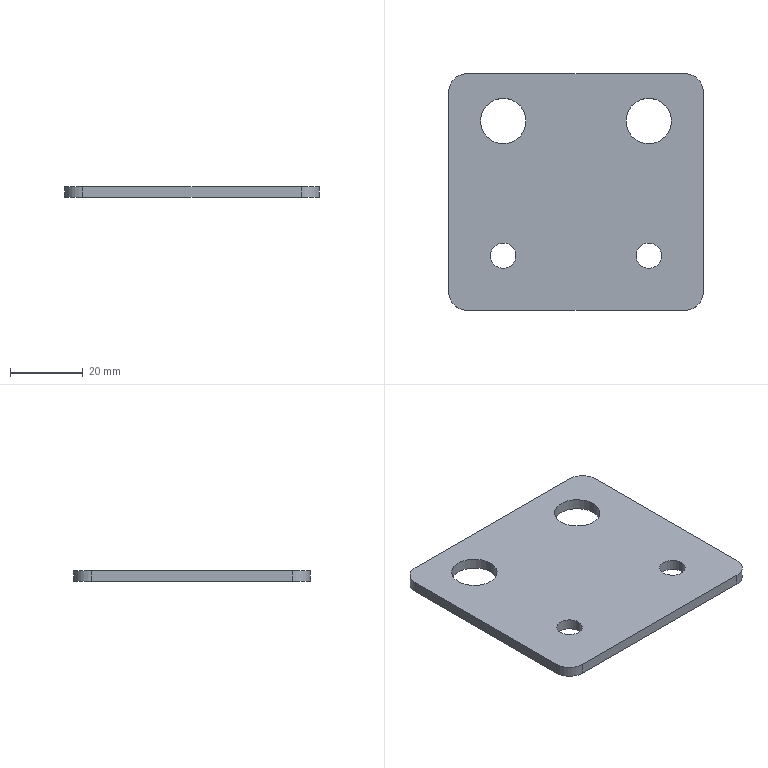Part | STEP file | Sensor mounting plate | 1 solid | 18 faces | box 70 x 65 x 3 mm | volume 12618 mm3 | cylinder 12 | plane 6 | commonest cylinder face diameters 7 x4 10 x4 12.5 x4
STEP:
#1=CARTESIAN_POINT('',(0.,0.,0.));
#2=DIRECTION('',(0.,0.,1.));
#3=DIRECTION('',(1.,0.,0.));
#4=AXIS2_PLACEMENT_3D('',#1,#2,#3);
#5=CARTESIAN_POINT('',(-16.5,-17.5,0.));
#6=VERTEX_POINT('',#5);
#7=CARTESIAN_POINT('',(-16.5,-17.5,3.));
#8=VERTEX_POINT('',#7);
#9=CARTESIAN_POINT('',(-16.5,-17.5,3.));
#10=DIRECTION('',(0.,0.,1.));
#11=VECTOR('',#10,1.);
#12=LINE('',#9,#11);
#13=CARTESIAN_POINT('',(-20.,-17.5,3.));
#14=DIRECTION('',(0.,0.,1.));
#15=DIRECTION('',(1.,0.,0.));
#16=AXIS2_PLACEMENT_3D('',#13,#14,#15);
#17=CYLINDRICAL_SURFACE('',#16,3.5);
#18=CARTESIAN_POINT('',(6.283,0.));
#19=DIRECTION('',(0.,1.));
#20=VECTOR('',#19,1.);
#21=LINE('',#18,#20);
#22=(GEOMETRIC_REPRESENTATION_CONTEXT(2)PARAMETRIC_REPRESENTATION_CONTEXT()REPRESENTATION_CONTEXT('',''));
#23=DEFINITIONAL_REPRESENTATION('',(#21),#22);
#24=PCURVE('',#17,#23);
#25=CARTESIAN_POINT('',(-20.,-17.5,3.));
#26=DIRECTION('',(0.,0.,1.));
#27=DIRECTION('',(1.,0.,0.));
#28=AXIS2_PLACEMENT_3D('',#25,#26,#27);
#29=CYLINDRICAL_SURFACE('',#28,3.5);
#30=CARTESIAN_POINT('',(0.,0.));
#31=DIRECTION('',(0.,1.));
#32=VECTOR('',#31,1.);
#33=LINE('',#30,#32);
#34=(GEOMETRIC_REPRESENTATION_CONTEXT(2)PARAMETRIC_REPRESENTATION_CONTEXT()REPRESENTATION_CONTEXT('',''));
#35=DEFINITIONAL_REPRESENTATION('',(#33),#34);
#36=PCURVE('',#29,#35);
#37=SURFACE_CURVE('',#12,(#24,#36),.PCURVE_S1.);
#38=EDGE_CURVE('',#6,#8,#37,.T.);
#39=ORIENTED_EDGE('',*,*,#38,.T.);
#40=CARTESIAN_POINT('',(-23.5,-17.5,3.));
#41=VERTEX_POINT('',#40);
#42=CARTESIAN_POINT('',(-20.,-17.5,3.));
#43=DIRECTION('',(0.,0.,1.));
#44=DIRECTION('',(1.,0.,0.));
#45=AXIS2_PLACEMENT_3D('',#42,#43,#44);
#46=CIRCLE('',#45,3.5);
#47=CARTESIAN_POINT('',(0.,0.));
#48=DIRECTION('',(1.,0.));
#49=VECTOR('',#48,1.);
#50=LINE('',#47,#49);
#51=(GEOMETRIC_REPRESENTATION_CONTEXT(2)PARAMETRIC_REPRESENTATION_CONTEXT()REPRESENTATION_CONTEXT('',''));
#52=DEFINITIONAL_REPRESENTATION('',(#50),#51);
#53=PCURVE('',#17,#52);
#54=CARTESIAN_POINT('',(0.,0.,3.));
#55=DIRECTION('',(0.,0.,1.));
#56=DIRECTION('',(1.,0.,0.));
#57=AXIS2_PLACEMENT_3D('',#54,#55,#56);
#58=PLANE('',#57);
#59=CARTESIAN_POINT('',(-20.,-17.5));
#60=DIRECTION('',(1.,0.));
#61=AXIS2_PLACEMENT_2D('',#59,#60);
#62=CIRCLE('',#61,3.5);
#63=(GEOMETRIC_REPRESENTATION_CONTEXT(2)PARAMETRIC_REPRESENTATION_CONTEXT()REPRESENTATION_CONTEXT('',''));
#64=DEFINITIONAL_REPRESENTATION('',(#62),#63);
#65=PCURVE('',#58,#64);
#66=SURFACE_CURVE('',#46,(#53,#65),.PCURVE_S1.);
#67=EDGE_CURVE('',#41,#8,#66,.T.);
#68=ORIENTED_EDGE('',*,*,#67,.F.);
#69=CARTESIAN_POINT('',(-23.5,-17.5,0.));
#70=VERTEX_POINT('',#69);
#71=CARTESIAN_POINT('',(-23.5,-17.5,3.));
#72=DIRECTION('',(0.,0.,1.));
#73=VECTOR('',#72,1.);
#74=LINE('',#71,#73);
#75=CARTESIAN_POINT('',(3.142,0.));
#76=DIRECTION('',(0.,1.));
#77=VECTOR('',#76,1.);
#78=LINE('',#75,#77);
#79=(GEOMETRIC_REPRESENTATION_CONTEXT(2)PARAMETRIC_REPRESENTATION_CONTEXT()REPRESENTATION_CONTEXT('',''));
#80=DEFINITIONAL_REPRESENTATION('',(#78),#79);
#81=PCURVE('',#17,#80);
#82=CARTESIAN_POINT('',(3.142,0.));
#83=DIRECTION('',(0.,1.));
#84=VECTOR('',#83,1.);
#85=LINE('',#82,#84);
#86=(GEOMETRIC_REPRESENTATION_CONTEXT(2)PARAMETRIC_REPRESENTATION_CONTEXT()REPRESENTATION_CONTEXT('',''));
#87=DEFINITIONAL_REPRESENTATION('',(#85),#86);
#88=PCURVE('',#29,#87);
#89=SURFACE_CURVE('',#74,(#81,#88),.PCURVE_S1.);
#90=EDGE_CURVE('',#70,#41,#89,.T.);
#91=ORIENTED_EDGE('',*,*,#90,.F.);
#92=CARTESIAN_POINT('',(-20.,-17.5,0.));
#93=DIRECTION('',(0.,0.,1.));
#94=DIRECTION('',(1.,0.,0.));
#95=AXIS2_PLACEMENT_3D('',#92,#93,#94);
#96=CIRCLE('',#95,3.5);
#97=CARTESIAN_POINT('',(0.,-3.));
#98=DIRECTION('',(1.,0.));
#99=VECTOR('',#98,1.);
#100=LINE('',#97,#99);
#101=(GEOMETRIC_REPRESENTATION_CONTEXT(2)PARAMETRIC_REPRESENTATION_CONTEXT()REPRESENTATION_CONTEXT('',''));
#102=DEFINITIONAL_REPRESENTATION('',(#100),#101);
#103=PCURVE('',#17,#102);
#104=CARTESIAN_POINT('',(0.,0.,0.));
#105=DIRECTION('',(0.,0.,1.));
#106=DIRECTION('',(1.,0.,0.));
#107=AXIS2_PLACEMENT_3D('',#104,#105,#106);
#108=PLANE('',#107);
#109=CARTESIAN_POINT('',(-20.,-17.5));
#110=DIRECTION('',(1.,0.));
#111=AXIS2_PLACEMENT_2D('',#109,#110);
#112=CIRCLE('',#111,3.5);
#113=(GEOMETRIC_REPRESENTATION_CONTEXT(2)PARAMETRIC_REPRESENTATION_CONTEXT()REPRESENTATION_CONTEXT('',''));
#114=DEFINITIONAL_REPRESENTATION('',(#112),#113);
#115=PCURVE('',#108,#114);
#116=SURFACE_CURVE('',#96,(#103,#115),.PCURVE_S1.);
#117=EDGE_CURVE('',#70,#6,#116,.T.);
#118=ORIENTED_EDGE('',*,*,#117,.T.);
#119=EDGE_LOOP('',(#39,#68,#91,#118));
#120=FACE_BOUND('',#119,.F.);
#121=ADVANCED_FACE('',(#120),#17,.F.);
#122=CARTESIAN_POINT('',(23.5,-17.5,0.));
#123=VERTEX_POINT('',#122);
#124=CARTESIAN_POINT('',(23.5,-17.5,3.));
#125=VERTEX_POINT('',#124);
#126=CARTESIAN_POINT('',(23.5,-17.5,3.));
#127=DIRECTION('',(0.,0.,1.));
#128=VECTOR('',#127,1.);
#129=LINE('',#126,#128);
#130=CARTESIAN_POINT('',(20.,-17.5,3.));
#131=DIRECTION('',(0.,0.,1.));
#132=DIRECTION('',(1.,0.,0.));
#133=AXIS2_PLACEMENT_3D('',#130,#131,#132);
#134=CYLINDRICAL_SURFACE('',#133,3.5);
#135=CARTESIAN_POINT('',(6.283,0.));
#136=DIRECTION('',(0.,1.));
#137=VECTOR('',#136,1.);
#138=LINE('',#135,#137);
#139=(GEOMETRIC_REPRESENTATION_CONTEXT(2)PARAMETRIC_REPRESENTATION_CONTEXT()REPRESENTATION_CONTEXT('',''));
#140=DEFINITIONAL_REPRESENTATION('',(#138),#139);
#141=PCURVE('',#134,#140);
#142=CARTESIAN_POINT('',(20.,-17.5,3.));
#143=DIRECTION('',(0.,0.,1.));
#144=DIRECTION('',(1.,0.,0.));
#145=AXIS2_PLACEMENT_3D('',#142,#143,#144);
#146=CYLINDRICAL_SURFACE('',#145,3.5);
#147=CARTESIAN_POINT('',(0.,0.));
#148=DIRECTION('',(0.,1.));
#149=VECTOR('',#148,1.);
#150=LINE('',#147,#149);
#151=(GEOMETRIC_REPRESENTATION_CONTEXT(2)PARAMETRIC_REPRESENTATION_CONTEXT()REPRESENTATION_CONTEXT('',''));
#152=DEFINITIONAL_REPRESENTATION('',(#150),#151);
#153=PCURVE('',#146,#152);
#154=SURFACE_CURVE('',#129,(#141,#153),.PCURVE_S1.);
#155=EDGE_CURVE('',#123,#125,#154,.T.);
#156=ORIENTED_EDGE('',*,*,#155,.T.);
#157=CARTESIAN_POINT('',(16.5,-17.5,3.));
#158=VERTEX_POINT('',#157);
#159=CARTESIAN_POINT('',(20.,-17.5,3.));
#160=DIRECTION('',(0.,0.,1.));
#161=DIRECTION('',(1.,0.,0.));
#162=AXIS2_PLACEMENT_3D('',#159,#160,#161);
#163=CIRCLE('',#162,3.5);
#164=CARTESIAN_POINT('',(0.,0.));
#165=DIRECTION('',(1.,0.));
#166=VECTOR('',#165,1.);
#167=LINE('',#164,#166);
#168=(GEOMETRIC_REPRESENTATION_CONTEXT(2)PARAMETRIC_REPRESENTATION_CONTEXT()REPRESENTATION_CONTEXT('',''));
#169=DEFINITIONAL_REPRESENTATION('',(#167),#168);
#170=PCURVE('',#134,#169);
#171=CARTESIAN_POINT('',(20.,-17.5));
#172=DIRECTION('',(1.,0.));
#173=AXIS2_PLACEMENT_2D('',#171,#172);
#174=CIRCLE('',#173,3.5);
#175=(GEOMETRIC_REPRESENTATION_CONTEXT(2)PARAMETRIC_REPRESENTATION_CONTEXT()REPRESENTATION_CONTEXT('',''));
#176=DEFINITIONAL_REPRESENTATION('',(#174),#175);
#177=PCURVE('',#58,#176);
#178=SURFACE_CURVE('',#163,(#170,#177),.PCURVE_S1.);
#179=EDGE_CURVE('',#158,#125,#178,.T.);
#180=ORIENTED_EDGE('',*,*,#179,.F.);
#181=CARTESIAN_POINT('',(16.5,-17.5,0.));
#182=VERTEX_POINT('',#181);
#183=CARTESIAN_POINT('',(16.5,-17.5,3.));
#184=DIRECTION('',(0.,0.,1.));
#185=VECTOR('',#184,1.);
#186=LINE('',#183,#185);
#187=CARTESIAN_POINT('',(3.142,0.));
#188=DIRECTION('',(0.,1.));
#189=VECTOR('',#188,1.);
#190=LINE('',#187,#189);
#191=(GEOMETRIC_REPRESENTATION_CONTEXT(2)PARAMETRIC_REPRESENTATION_CONTEXT()REPRESENTATION_CONTEXT('',''));
#192=DEFINITIONAL_REPRESENTATION('',(#190),#191);
#193=PCURVE('',#134,#192);
#194=CARTESIAN_POINT('',(3.142,0.));
#195=DIRECTION('',(0.,1.));
#196=VECTOR('',#195,1.);
#197=LINE('',#194,#196);
#198=(GEOMETRIC_REPRESENTATION_CONTEXT(2)PARAMETRIC_REPRESENTATION_CONTEXT()REPRESENTATION_CONTEXT('',''));
#199=DEFINITIONAL_REPRESENTATION('',(#197),#198);
#200=PCURVE('',#146,#199);
#201=SURFACE_CURVE('',#186,(#193,#200),.PCURVE_S1.);
#202=EDGE_CURVE('',#182,#158,#201,.T.);
#203=ORIENTED_EDGE('',*,*,#202,.F.);
#204=CARTESIAN_POINT('',(20.,-17.5,0.));
#205=DIRECTION('',(0.,0.,1.));
#206=DIRECTION('',(1.,0.,0.));
#207=AXIS2_PLACEMENT_3D('',#204,#205,#206);
#208=CIRCLE('',#207,3.5);
#209=CARTESIAN_POINT('',(0.,-3.));
#210=DIRECTION('',(1.,0.));
#211=VECTOR('',#210,1.);
#212=LINE('',#209,#211);
#213=(GEOMETRIC_REPRESENTATION_CONTEXT(2)PARAMETRIC_REPRESENTATION_CONTEXT()REPRESENTATION_CONTEXT('',''));
#214=DEFINITIONAL_REPRESENTATION('',(#212),#213);
#215=PCURVE('',#134,#214);
#216=CARTESIAN_POINT('',(20.,-17.5));
#217=DIRECTION('',(1.,0.));
#218=AXIS2_PLACEMENT_2D('',#216,#217);
#219=CIRCLE('',#218,3.5);
#220=(GEOMETRIC_REPRESENTATION_CONTEXT(2)PARAMETRIC_REPRESENTATION_CONTEXT()REPRESENTATION_CONTEXT('',''));
#221=DEFINITIONAL_REPRESENTATION('',(#219),#220);
#222=PCURVE('',#108,#221);
#223=SURFACE_CURVE('',#208,(#215,#222),.PCURVE_S1.);
#224=EDGE_CURVE('',#182,#123,#223,.T.);
#225=ORIENTED_EDGE('',*,*,#224,.T.);
#226=EDGE_LOOP('',(#156,#180,#203,#225));
#227=FACE_BOUND('',#226,.F.);
#228=ADVANCED_FACE('',(#227),#134,.F.);
#229=CARTESIAN_POINT('',(26.25,19.5,0.));
#230=VERTEX_POINT('',#229);
#231=CARTESIAN_POINT('',(26.25,19.5,3.));
#232=VERTEX_POINT('',#231);
#233=CARTESIAN_POINT('',(26.25,19.5,0.));
#234=DIRECTION('',(0.,0.,1.));
#235=VECTOR('',#234,1.);
#236=LINE('',#233,#235);
#237=CARTESIAN_POINT('',(20.,19.5,0.));
#238=DIRECTION('',(0.,0.,1.));
#239=DIRECTION('',(1.,0.,0.));
#240=AXIS2_PLACEMENT_3D('',#237,#238,#239);
#241=CYLINDRICAL_SURFACE('',#240,6.25);
#242=CARTESIAN_POINT('',(6.283,0.));
#243=DIRECTION('',(0.,1.));
#244=VECTOR('',#243,1.);
#245=LINE('',#242,#244);
#246=(GEOMETRIC_REPRESENTATION_CONTEXT(2)PARAMETRIC_REPRESENTATION_CONTEXT()REPRESENTATION_CONTEXT('',''));
#247=DEFINITIONAL_REPRESENTATION('',(#245),#246);
#248=PCURVE('',#241,#247);
#249=CARTESIAN_POINT('',(20.,19.5,0.));
#250=DIRECTION('',(0.,0.,1.));
#251=DIRECTION('',(1.,0.,0.));
#252=AXIS2_PLACEMENT_3D('',#249,#250,#251);
#253=CYLINDRICAL_SURFACE('',#252,6.25);
#254=CARTESIAN_POINT('',(0.,0.));
#255=DIRECTION('',(0.,1.));
#256=VECTOR('',#255,1.);
#257=LINE('',#254,#256);
#258=(GEOMETRIC_REPRESENTATION_CONTEXT(2)PARAMETRIC_REPRESENTATION_CONTEXT()REPRESENTATION_CONTEXT('',''));
#259=DEFINITIONAL_REPRESENTATION('',(#257),#258);
#260=PCURVE('',#253,#259);
#261=SURFACE_CURVE('',#236,(#248,#260),.PCURVE_S1.);
#262=EDGE_CURVE('',#230,#232,#261,.T.);
#263=ORIENTED_EDGE('',*,*,#262,.T.);
#264=CARTESIAN_POINT('',(13.75,19.5,3.));
#265=VERTEX_POINT('',#264);
#266=CARTESIAN_POINT('',(20.,19.5,3.));
#267=DIRECTION('',(0.,0.,1.));
#268=DIRECTION('',(1.,0.,0.));
#269=AXIS2_PLACEMENT_3D('',#266,#267,#268);
#270=CIRCLE('',#269,6.25);
#271=CARTESIAN_POINT('',(0.,3.));
#272=DIRECTION('',(1.,0.));
#273=VECTOR('',#272,1.);
#274=LINE('',#271,#273);
#275=(GEOMETRIC_REPRESENTATION_CONTEXT(2)PARAMETRIC_REPRESENTATION_CONTEXT()REPRESENTATION_CONTEXT('',''));
#276=DEFINITIONAL_REPRESENTATION('',(#274),#275);
#277=PCURVE('',#241,#276);
#278=CARTESIAN_POINT('',(20.,19.5));
#279=DIRECTION('',(1.,0.));
#280=AXIS2_PLACEMENT_2D('',#278,#279);
#281=CIRCLE('',#280,6.25);
#282=(GEOMETRIC_REPRESENTATION_CONTEXT(2)PARAMETRIC_REPRESENTATION_CONTEXT()REPRESENTATION_CONTEXT('',''));
#283=DEFINITIONAL_REPRESENTATION('',(#281),#282);
#284=PCURVE('',#58,#283);
#285=SURFACE_CURVE('',#270,(#277,#284),.PCURVE_S1.);
#286=EDGE_CURVE('',#265,#232,#285,.T.);
#287=ORIENTED_EDGE('',*,*,#286,.F.);
#288=CARTESIAN_POINT('',(13.75,19.5,0.));
#289=VERTEX_POINT('',#288);
#290=CARTESIAN_POINT('',(13.75,19.5,0.));
#291=DIRECTION('',(0.,0.,1.));
#292=VECTOR('',#291,1.);
#293=LINE('',#290,#292);
#294=CARTESIAN_POINT('',(3.142,0.));
#295=DIRECTION('',(0.,1.));
#296=VECTOR('',#295,1.);
#297=LINE('',#294,#296);
#298=(GEOMETRIC_REPRESENTATION_CONTEXT(2)PARAMETRIC_REPRESENTATION_CONTEXT()REPRESENTATION_CONTEXT('',''));
#299=DEFINITIONAL_REPRESENTATION('',(#297),#298);
#300=PCURVE('',#241,#299);
#301=CARTESIAN_POINT('',(3.142,0.));
#302=DIRECTION('',(0.,1.));
#303=VECTOR('',#302,1.);
#304=LINE('',#301,#303);
#305=(GEOMETRIC_REPRESENTATION_CONTEXT(2)PARAMETRIC_REPRESENTATION_CONTEXT()REPRESENTATION_CONTEXT('',''));
#306=DEFINITIONAL_REPRESENTATION('',(#304),#305);
#307=PCURVE('',#253,#306);
#308=SURFACE_CURVE('',#293,(#300,#307),.PCURVE_S1.);
#309=EDGE_CURVE('',#289,#265,#308,.T.);
#310=ORIENTED_EDGE('',*,*,#309,.F.);
#311=CARTESIAN_POINT('',(20.,19.5,0.));
#312=DIRECTION('',(0.,0.,1.));
#313=DIRECTION('',(1.,0.,0.));
#314=AXIS2_PLACEMENT_3D('',#311,#312,#313);
#315=CIRCLE('',#314,6.25);
#316=CARTESIAN_POINT('',(0.,0.));
#317=DIRECTION('',(1.,0.));
#318=VECTOR('',#317,1.);
#319=LINE('',#316,#318);
#320=(GEOMETRIC_REPRESENTATION_CONTEXT(2)PARAMETRIC_REPRESENTATION_CONTEXT()REPRESENTATION_CONTEXT('',''));
#321=DEFINITIONAL_REPRESENTATION('',(#319),#320);
#322=PCURVE('',#241,#321);
#323=CARTESIAN_POINT('',(20.,19.5));
#324=DIRECTION('',(1.,0.));
#325=AXIS2_PLACEMENT_2D('',#323,#324);
#326=CIRCLE('',#325,6.25);
#327=(GEOMETRIC_REPRESENTATION_CONTEXT(2)PARAMETRIC_REPRESENTATION_CONTEXT()REPRESENTATION_CONTEXT('',''));
#328=DEFINITIONAL_REPRESENTATION('',(#326),#327);
#329=PCURVE('',#108,#328);
#330=SURFACE_CURVE('',#315,(#322,#329),.PCURVE_S1.);
#331=EDGE_CURVE('',#289,#230,#330,.T.);
#332=ORIENTED_EDGE('',*,*,#331,.T.);
#333=EDGE_LOOP('',(#263,#287,#310,#332));
#334=FACE_BOUND('',#333,.F.);
#335=ADVANCED_FACE('',(#334),#241,.F.);
#336=CARTESIAN_POINT('',(-13.75,19.5,0.));
#337=VERTEX_POINT('',#336);
#338=CARTESIAN_POINT('',(-13.75,19.5,3.));
#339=VERTEX_POINT('',#338);
#340=CARTESIAN_POINT('',(-13.75,19.5,0.));
#341=DIRECTION('',(0.,0.,1.));
#342=VECTOR('',#341,1.);
#343=LINE('',#340,#342);
#344=CARTESIAN_POINT('',(-20.,19.5,0.));
#345=DIRECTION('',(0.,0.,1.));
#346=DIRECTION('',(1.,0.,0.));
#347=AXIS2_PLACEMENT_3D('',#344,#345,#346);
#348=CYLINDRICAL_SURFACE('',#347,6.25);
#349=CARTESIAN_POINT('',(6.283,0.));
#350=DIRECTION('',(0.,1.));
#351=VECTOR('',#350,1.);
#352=LINE('',#349,#351);
#353=(GEOMETRIC_REPRESENTATION_CONTEXT(2)PARAMETRIC_REPRESENTATION_CONTEXT()REPRESENTATION_CONTEXT('',''));
#354=DEFINITIONAL_REPRESENTATION('',(#352),#353);
#355=PCURVE('',#348,#354);
#356=CARTESIAN_POINT('',(-20.,19.5,0.));
#357=DIRECTION('',(0.,0.,1.));
#358=DIRECTION('',(1.,0.,0.));
#359=AXIS2_PLACEMENT_3D('',#356,#357,#358);
#360=CYLINDRICAL_SURFACE('',#359,6.25);
#361=CARTESIAN_POINT('',(0.,0.));
#362=DIRECTION('',(0.,1.));
#363=VECTOR('',#362,1.);
#364=LINE('',#361,#363);
#365=(GEOMETRIC_REPRESENTATION_CONTEXT(2)PARAMETRIC_REPRESENTATION_CONTEXT()REPRESENTATION_CONTEXT('',''));
#366=DEFINITIONAL_REPRESENTATION('',(#364),#365);
#367=PCURVE('',#360,#366);
#368=SURFACE_CURVE('',#343,(#355,#367),.PCURVE_S1.);
#369=EDGE_CURVE('',#337,#339,#368,.T.);
#370=ORIENTED_EDGE('',*,*,#369,.T.);
#371=CARTESIAN_POINT('',(-26.25,19.5,3.));
#372=VERTEX_POINT('',#371);
#373=CARTESIAN_POINT('',(-20.,19.5,3.));
#374=DIRECTION('',(0.,0.,1.));
#375=DIRECTION('',(1.,0.,0.));
#376=AXIS2_PLACEMENT_3D('',#373,#374,#375);
#377=CIRCLE('',#376,6.25);
#378=CARTESIAN_POINT('',(0.,3.));
#379=DIRECTION('',(1.,0.));
#380=VECTOR('',#379,1.);
#381=LINE('',#378,#380);
#382=(GEOMETRIC_REPRESENTATION_CONTEXT(2)PARAMETRIC_REPRESENTATION_CONTEXT()REPRESENTATION_CONTEXT('',''));
#383=DEFINITIONAL_REPRESENTATION('',(#381),#382);
#384=PCURVE('',#348,#383);
#385=CARTESIAN_POINT('',(-20.,19.5));
#386=DIRECTION('',(1.,0.));
#387=AXIS2_PLACEMENT_2D('',#385,#386);
#388=CIRCLE('',#387,6.25);
#389=(GEOMETRIC_REPRESENTATION_CONTEXT(2)PARAMETRIC_REPRESENTATION_CONTEXT()REPRESENTATION_CONTEXT('',''));
#390=DEFINITIONAL_REPRESENTATION('',(#388),#389);
#391=PCURVE('',#58,#390);
#392=SURFACE_CURVE('',#377,(#384,#391),.PCURVE_S1.);
#393=EDGE_CURVE('',#372,#339,#392,.T.);
#394=ORIENTED_EDGE('',*,*,#393,.F.);
#395=CARTESIAN_POINT('',(-26.25,19.5,0.));
#396=VERTEX_POINT('',#395);
#397=CARTESIAN_POINT('',(-26.25,19.5,0.));
#398=DIRECTION('',(0.,0.,1.));
#399=VECTOR('',#398,1.);
#400=LINE('',#397,#399);
#401=CARTESIAN_POINT('',(3.142,0.));
#402=DIRECTION('',(0.,1.));
#403=VECTOR('',#402,1.);
#404=LINE('',#401,#403);
#405=(GEOMETRIC_REPRESENTATION_CONTEXT(2)PARAMETRIC_REPRESENTATION_CONTEXT()REPRESENTATION_CONTEXT('',''));
#406=DEFINITIONAL_REPRESENTATION('',(#404),#405);
#407=PCURVE('',#348,#406);
#408=CARTESIAN_POINT('',(3.142,0.));
#409=DIRECTION('',(0.,1.));
#410=VECTOR('',#409,1.);
#411=LINE('',#408,#410);
#412=(GEOMETRIC_REPRESENTATION_CONTEXT(2)PARAMETRIC_REPRESENTATION_CONTEXT()REPRESENTATION_CONTEXT('',''));
#413=DEFINITIONAL_REPRESENTATION('',(#411),#412);
#414=PCURVE('',#360,#413);
#415=SURFACE_CURVE('',#400,(#407,#414),.PCURVE_S1.);
#416=EDGE_CURVE('',#396,#372,#415,.T.);
#417=ORIENTED_EDGE('',*,*,#416,.F.);
#418=CARTESIAN_POINT('',(-20.,19.5,0.));
#419=DIRECTION('',(0.,0.,1.));
#420=DIRECTION('',(1.,0.,0.));
#421=AXIS2_PLACEMENT_3D('',#418,#419,#420);
#422=CIRCLE('',#421,6.25);
#423=CARTESIAN_POINT('',(0.,0.));
#424=DIRECTION('',(1.,0.));
#425=VECTOR('',#424,1.);
#426=LINE('',#423,#425);
#427=(GEOMETRIC_REPRESENTATION_CONTEXT(2)PARAMETRIC_REPRESENTATION_CONTEXT()REPRESENTATION_CONTEXT('',''));
#428=DEFINITIONAL_REPRESENTATION('',(#426),#427);
#429=PCURVE('',#348,#428);
#430=CARTESIAN_POINT('',(-20.,19.5));
#431=DIRECTION('',(1.,0.));
#432=AXIS2_PLACEMENT_2D('',#430,#431);
#433=CIRCLE('',#432,6.25);
#434=(GEOMETRIC_REPRESENTATION_CONTEXT(2)PARAMETRIC_REPRESENTATION_CONTEXT()REPRESENTATION_CONTEXT('',''));
#435=DEFINITIONAL_REPRESENTATION('',(#433),#434);
#436=PCURVE('',#108,#435);
#437=SURFACE_CURVE('',#422,(#429,#436),.PCURVE_S1.);
#438=EDGE_CURVE('',#396,#337,#437,.T.);
#439=ORIENTED_EDGE('',*,*,#438,.T.);
#440=EDGE_LOOP('',(#370,#394,#417,#439));
#441=FACE_BOUND('',#440,.F.);
#442=ADVANCED_FACE('',(#441),#348,.F.);
#443=CARTESIAN_POINT('',(35.,-27.5,3.));
#444=VERTEX_POINT('',#443);
#445=CARTESIAN_POINT('',(35.,27.5,3.));
#446=VERTEX_POINT('',#445);
#447=CARTESIAN_POINT('',(35.,32.5,3.));
#448=DIRECTION('',(0.,1.,0.));
#449=VECTOR('',#448,1.);
#450=LINE('',#447,#449);
#451=CARTESIAN_POINT('',(35.,32.5,3.));
#452=DIRECTION('',(-1.,0.,0.));
#453=DIRECTION('',(0.,-1.,0.));
#454=AXIS2_PLACEMENT_3D('',#451,#452,#453);
#455=PLANE('',#454);
#456=CARTESIAN_POINT('',(0.,0.));
#457=DIRECTION('',(-1.,0.));
#458=VECTOR('',#457,1.);
#459=LINE('',#456,#458);
#460=(GEOMETRIC_REPRESENTATION_CONTEXT(2)PARAMETRIC_REPRESENTATION_CONTEXT()REPRESENTATION_CONTEXT('',''));
#461=DEFINITIONAL_REPRESENTATION('',(#459),#460);
#462=PCURVE('',#455,#461);
#463=CARTESIAN_POINT('',(35.,32.5));
#464=DIRECTION('',(0.,1.));
#465=VECTOR('',#464,1.);
#466=LINE('',#463,#465);
#467=(GEOMETRIC_REPRESENTATION_CONTEXT(2)PARAMETRIC_REPRESENTATION_CONTEXT()REPRESENTATION_CONTEXT('',''));
#468=DEFINITIONAL_REPRESENTATION('',(#466),#467);
#469=PCURVE('',#58,#468);
#470=SURFACE_CURVE('',#450,(#462,#469),.PCURVE_S1.);
#471=EDGE_CURVE('',#444,#446,#470,.T.);
#472=ORIENTED_EDGE('',*,*,#471,.F.);
#473=CARTESIAN_POINT('',(35.,-27.5,0.));
#474=VERTEX_POINT('',#473);
#475=CARTESIAN_POINT('',(35.,-27.5,3.));
#476=DIRECTION('',(0.,0.,-1.));
#477=VECTOR('',#476,1.);
#478=LINE('',#475,#477);
#479=CARTESIAN_POINT('',(60.,0.));
#480=DIRECTION('',(0.,-1.));
#481=VECTOR('',#480,1.);
#482=LINE('',#479,#481);
#483=(GEOMETRIC_REPRESENTATION_CONTEXT(2)PARAMETRIC_REPRESENTATION_CONTEXT()REPRESENTATION_CONTEXT('',''));
#484=DEFINITIONAL_REPRESENTATION('',(#482),#483);
#485=PCURVE('',#455,#484);
#486=CARTESIAN_POINT('',(30.,-27.5,3.));
#487=DIRECTION('',(0.,0.,-1.));
#488=DIRECTION('',(-1.,0.,0.));
#489=AXIS2_PLACEMENT_3D('',#486,#487,#488);
#490=CYLINDRICAL_SURFACE('',#489,5.);
#491=CARTESIAN_POINT('',(3.142,0.));
#492=DIRECTION('',(0.,1.));
#493=VECTOR('',#492,1.);
#494=LINE('',#491,#493);
#495=(GEOMETRIC_REPRESENTATION_CONTEXT(2)PARAMETRIC_REPRESENTATION_CONTEXT()REPRESENTATION_CONTEXT('',''));
#496=DEFINITIONAL_REPRESENTATION('',(#494),#495);
#497=PCURVE('',#490,#496);
#498=SURFACE_CURVE('',#478,(#485,#497),.PCURVE_S1.);
#499=EDGE_CURVE('',#444,#474,#498,.T.);
#500=ORIENTED_EDGE('',*,*,#499,.T.);
#501=CARTESIAN_POINT('',(35.,27.5,0.));
#502=VERTEX_POINT('',#501);
#503=CARTESIAN_POINT('',(35.,32.5,0.));
#504=DIRECTION('',(0.,1.,0.));
#505=VECTOR('',#504,1.);
#506=LINE('',#503,#505);
#507=CARTESIAN_POINT('',(0.,-3.));
#508=DIRECTION('',(-1.,0.));
#509=VECTOR('',#508,1.);
#510=LINE('',#507,#509);
#511=(GEOMETRIC_REPRESENTATION_CONTEXT(2)PARAMETRIC_REPRESENTATION_CONTEXT()REPRESENTATION_CONTEXT('',''));
#512=DEFINITIONAL_REPRESENTATION('',(#510),#511);
#513=PCURVE('',#455,#512);
#514=CARTESIAN_POINT('',(35.,32.5));
#515=DIRECTION('',(0.,1.));
#516=VECTOR('',#515,1.);
#517=LINE('',#514,#516);
#518=(GEOMETRIC_REPRESENTATION_CONTEXT(2)PARAMETRIC_REPRESENTATION_CONTEXT()REPRESENTATION_CONTEXT('',''));
#519=DEFINITIONAL_REPRESENTATION('',(#517),#518);
#520=PCURVE('',#108,#519);
#521=SURFACE_CURVE('',#506,(#513,#520),.PCURVE_S1.);
#522=EDGE_CURVE('',#474,#502,#521,.T.);
#523=ORIENTED_EDGE('',*,*,#522,.T.);
#524=CARTESIAN_POINT('',(35.,27.5,3.));
#525=DIRECTION('',(0.,0.,1.));
#526=VECTOR('',#525,1.);
#527=LINE('',#524,#526);
#528=CARTESIAN_POINT('',(5.,0.));
#529=DIRECTION('',(0.,1.));
#530=VECTOR('',#529,1.);
#531=LINE('',#528,#530);
#532=(GEOMETRIC_REPRESENTATION_CONTEXT(2)PARAMETRIC_REPRESENTATION_CONTEXT()REPRESENTATION_CONTEXT('',''));
#533=DEFINITIONAL_REPRESENTATION('',(#531),#532);
#534=PCURVE('',#455,#533);
#535=CARTESIAN_POINT('',(30.,27.5,3.));
#536=DIRECTION('',(0.,0.,-1.));
#537=DIRECTION('',(-1.,0.,0.));
#538=AXIS2_PLACEMENT_3D('',#535,#536,#537);
#539=CYLINDRICAL_SURFACE('',#538,5.);
#540=CARTESIAN_POINT('',(3.142,0.));
#541=DIRECTION('',(0.,-1.));
#542=VECTOR('',#541,1.);
#543=LINE('',#540,#542);
#544=(GEOMETRIC_REPRESENTATION_CONTEXT(2)PARAMETRIC_REPRESENTATION_CONTEXT()REPRESENTATION_CONTEXT('',''));
#545=DEFINITIONAL_REPRESENTATION('',(#543),#544);
#546=PCURVE('',#539,#545);
#547=SURFACE_CURVE('',#527,(#534,#546),.PCURVE_S1.);
#548=EDGE_CURVE('',#502,#446,#547,.T.);
#549=ORIENTED_EDGE('',*,*,#548,.T.);
#550=EDGE_LOOP('',(#472,#500,#523,#549));
#551=FACE_BOUND('',#550,.T.);
#552=ADVANCED_FACE('',(#551),#455,.F.);
#553=CARTESIAN_POINT('',(30.,32.5,3.));
#554=VERTEX_POINT('',#553);
#555=CARTESIAN_POINT('',(-30.,32.5,3.));
#556=VERTEX_POINT('',#555);
#557=CARTESIAN_POINT('',(-35.,32.5,3.));
#558=DIRECTION('',(-1.,0.,0.));
#559=VECTOR('',#558,1.);
#560=LINE('',#557,#559);
#561=CARTESIAN_POINT('',(-35.,32.5,3.));
#562=DIRECTION('',(0.,-1.,0.));
#563=DIRECTION('',(0.,0.,-1.));
#564=AXIS2_PLACEMENT_3D('',#561,#562,#563);
#565=PLANE('',#564);
#566=CARTESIAN_POINT('',(0.,0.));
#567=DIRECTION('',(0.,-1.));
#568=VECTOR('',#567,1.);
#569=LINE('',#566,#568);
#570=(GEOMETRIC_REPRESENTATION_CONTEXT(2)PARAMETRIC_REPRESENTATION_CONTEXT()REPRESENTATION_CONTEXT('',''));
#571=DEFINITIONAL_REPRESENTATION('',(#569),#570);
#572=PCURVE('',#565,#571);
#573=CARTESIAN_POINT('',(-35.,32.5));
#574=DIRECTION('',(-1.,0.));
#575=VECTOR('',#574,1.);
#576=LINE('',#573,#575);
#577=(GEOMETRIC_REPRESENTATION_CONTEXT(2)PARAMETRIC_REPRESENTATION_CONTEXT()REPRESENTATION_CONTEXT('',''));
#578=DEFINITIONAL_REPRESENTATION('',(#576),#577);
#579=PCURVE('',#58,#578);
#580=SURFACE_CURVE('',#560,(#572,#579),.PCURVE_S1.);
#581=EDGE_CURVE('',#554,#556,#580,.T.);
#582=ORIENTED_EDGE('',*,*,#581,.F.);
#583=CARTESIAN_POINT('',(30.,32.5,0.));
#584=VERTEX_POINT('',#583);
#585=CARTESIAN_POINT('',(30.,32.5,3.));
#586=DIRECTION('',(0.,0.,-1.));
#587=VECTOR('',#586,1.);
#588=LINE('',#585,#587);
#589=CARTESIAN_POINT('',(0.,65.));
#590=DIRECTION('',(1.,0.));
#591=VECTOR('',#590,1.);
#592=LINE('',#589,#591);
#593=(GEOMETRIC_REPRESENTATION_CONTEXT(2)PARAMETRIC_REPRESENTATION_CONTEXT()REPRESENTATION_CONTEXT('',''));
#594=DEFINITIONAL_REPRESENTATION('',(#592),#593);
#595=PCURVE('',#565,#594);
#596=CARTESIAN_POINT('',(1.571,0.));
#597=DIRECTION('',(0.,1.));
#598=VECTOR('',#597,1.);
#599=LINE('',#596,#598);
#600=(GEOMETRIC_REPRESENTATION_CONTEXT(2)PARAMETRIC_REPRESENTATION_CONTEXT()REPRESENTATION_CONTEXT('',''));
#601=DEFINITIONAL_REPRESENTATION('',(#599),#600);
#602=PCURVE('',#539,#601);
#603=SURFACE_CURVE('',#588,(#595,#602),.PCURVE_S1.);
#604=EDGE_CURVE('',#554,#584,#603,.T.);
#605=ORIENTED_EDGE('',*,*,#604,.T.);
#606=CARTESIAN_POINT('',(-30.,32.5,0.));
#607=VERTEX_POINT('',#606);
#608=CARTESIAN_POINT('',(-35.,32.5,0.));
#609=DIRECTION('',(-1.,0.,0.));
#610=VECTOR('',#609,1.);
#611=LINE('',#608,#610);
#612=CARTESIAN_POINT('',(3.,0.));
#613=DIRECTION('',(0.,-1.));
#614=VECTOR('',#613,1.);
#615=LINE('',#612,#614);
#616=(GEOMETRIC_REPRESENTATION_CONTEXT(2)PARAMETRIC_REPRESENTATION_CONTEXT()REPRESENTATION_CONTEXT('',''));
#617=DEFINITIONAL_REPRESENTATION('',(#615),#616);
#618=PCURVE('',#565,#617);
#619=CARTESIAN_POINT('',(-35.,32.5));
#620=DIRECTION('',(-1.,0.));
#621=VECTOR('',#620,1.);
#622=LINE('',#619,#621);
#623=(GEOMETRIC_REPRESENTATION_CONTEXT(2)PARAMETRIC_REPRESENTATION_CONTEXT()REPRESENTATION_CONTEXT('',''));
#624=DEFINITIONAL_REPRESENTATION('',(#622),#623);
#625=PCURVE('',#108,#624);
#626=SURFACE_CURVE('',#611,(#618,#625),.PCURVE_S1.);
#627=EDGE_CURVE('',#584,#607,#626,.T.);
#628=ORIENTED_EDGE('',*,*,#627,.T.);
#629=CARTESIAN_POINT('',(-30.,32.5,3.));
#630=DIRECTION('',(0.,0.,1.));
#631=VECTOR('',#630,1.);
#632=LINE('',#629,#631);
#633=CARTESIAN_POINT('',(0.,5.));
#634=DIRECTION('',(-1.,0.));
#635=VECTOR('',#634,1.);
#636=LINE('',#633,#635);
#637=(GEOMETRIC_REPRESENTATION_CONTEXT(2)PARAMETRIC_REPRESENTATION_CONTEXT()REPRESENTATION_CONTEXT('',''));
#638=DEFINITIONAL_REPRESENTATION('',(#636),#637);
#639=PCURVE('',#565,#638);
#640=CARTESIAN_POINT('',(-30.,27.5,3.));
#641=DIRECTION('',(0.,0.,-1.));
#642=DIRECTION('',(-1.,0.,0.));
#643=AXIS2_PLACEMENT_3D('',#640,#641,#642);
#644=CYLINDRICAL_SURFACE('',#643,5.);
#645=CARTESIAN_POINT('',(1.571,0.));
#646=DIRECTION('',(0.,-1.));
#647=VECTOR('',#646,1.);
#648=LINE('',#645,#647);
#649=(GEOMETRIC_REPRESENTATION_CONTEXT(2)PARAMETRIC_REPRESENTATION_CONTEXT()REPRESENTATION_CONTEXT('',''));
#650=DEFINITIONAL_REPRESENTATION('',(#648),#649);
#651=PCURVE('',#644,#650);
#652=SURFACE_CURVE('',#632,(#639,#651),.PCURVE_S1.);
#653=EDGE_CURVE('',#607,#556,#652,.T.);
#654=ORIENTED_EDGE('',*,*,#653,.T.);
#655=EDGE_LOOP('',(#582,#605,#628,#654));
#656=FACE_BOUND('',#655,.T.);
#657=ADVANCED_FACE('',(#656),#565,.F.);
#658=CARTESIAN_POINT('',(-35.,27.5,0.));
#659=VERTEX_POINT('',#658);
#660=CARTESIAN_POINT('',(-35.,-27.5,0.));
#661=VERTEX_POINT('',#660);
#662=CARTESIAN_POINT('',(-35.,32.5,0.));
#663=DIRECTION('',(0.,-1.,0.));
#664=VECTOR('',#663,1.);
#665=LINE('',#662,#664);
#666=CARTESIAN_POINT('',(-35.,32.5,3.));
#667=DIRECTION('',(1.,0.,0.));
#668=DIRECTION('',(0.,0.,-1.));
#669=AXIS2_PLACEMENT_3D('',#666,#667,#668);
#670=PLANE('',#669);
#671=CARTESIAN_POINT('',(3.,0.));
#672=DIRECTION('',(0.,-1.));
#673=VECTOR('',#672,1.);
#674=LINE('',#671,#673);
#675=(GEOMETRIC_REPRESENTATION_CONTEXT(2)PARAMETRIC_REPRESENTATION_CONTEXT()REPRESENTATION_CONTEXT('',''));
#676=DEFINITIONAL_REPRESENTATION('',(#674),#675);
#677=PCURVE('',#670,#676);
#678=CARTESIAN_POINT('',(-35.,32.5));
#679=DIRECTION('',(0.,-1.));
#680=VECTOR('',#679,1.);
#681=LINE('',#678,#680);
#682=(GEOMETRIC_REPRESENTATION_CONTEXT(2)PARAMETRIC_REPRESENTATION_CONTEXT()REPRESENTATION_CONTEXT('',''));
#683=DEFINITIONAL_REPRESENTATION('',(#681),#682);
#684=PCURVE('',#108,#683);
#685=SURFACE_CURVE('',#665,(#677,#684),.PCURVE_S1.);
#686=EDGE_CURVE('',#659,#661,#685,.T.);
#687=ORIENTED_EDGE('',*,*,#686,.T.);
#688=CARTESIAN_POINT('',(-35.,-27.5,3.));
#689=VERTEX_POINT('',#688);
#690=CARTESIAN_POINT('',(-35.,-27.5,3.));
#691=DIRECTION('',(0.,0.,1.));
#692=VECTOR('',#691,1.);
#693=LINE('',#690,#692);
#694=CARTESIAN_POINT('',(0.,-60.));
#695=DIRECTION('',(-1.,0.));
#696=VECTOR('',#695,1.);
#697=LINE('',#694,#696);
#698=(GEOMETRIC_REPRESENTATION_CONTEXT(2)PARAMETRIC_REPRESENTATION_CONTEXT()REPRESENTATION_CONTEXT('',''));
#699=DEFINITIONAL_REPRESENTATION('',(#697),#698);
#700=PCURVE('',#670,#699);
#701=CARTESIAN_POINT('',(-30.,-27.5,3.));
#702=DIRECTION('',(0.,0.,-1.));
#703=DIRECTION('',(-1.,0.,0.));
#704=AXIS2_PLACEMENT_3D('',#701,#702,#703);
#705=CYLINDRICAL_SURFACE('',#704,5.);
#706=CARTESIAN_POINT('',(6.283,0.));
#707=DIRECTION('',(0.,-1.));
#708=VECTOR('',#707,1.);
#709=LINE('',#706,#708);
#710=(GEOMETRIC_REPRESENTATION_CONTEXT(2)PARAMETRIC_REPRESENTATION_CONTEXT()REPRESENTATION_CONTEXT('',''));
#711=DEFINITIONAL_REPRESENTATION('',(#709),#710);
#712=PCURVE('',#705,#711);
#713=SURFACE_CURVE('',#693,(#700,#712),.PCURVE_S1.);
#714=EDGE_CURVE('',#661,#689,#713,.T.);
#715=ORIENTED_EDGE('',*,*,#714,.T.);
#716=CARTESIAN_POINT('',(-35.,27.5,3.));
#717=VERTEX_POINT('',#716);
#718=CARTESIAN_POINT('',(-35.,32.5,3.));
#719=DIRECTION('',(0.,-1.,0.));
#720=VECTOR('',#719,1.);
#721=LINE('',#718,#720);
#722=CARTESIAN_POINT('',(0.,0.));
#723=DIRECTION('',(0.,-1.));
#724=VECTOR('',#723,1.);
#725=LINE('',#722,#724);
#726=(GEOMETRIC_REPRESENTATION_CONTEXT(2)PARAMETRIC_REPRESENTATION_CONTEXT()REPRESENTATION_CONTEXT('',''));
#727=DEFINITIONAL_REPRESENTATION('',(#725),#726);
#728=PCURVE('',#670,#727);
#729=CARTESIAN_POINT('',(-35.,32.5));
#730=DIRECTION('',(0.,-1.));
#731=VECTOR('',#730,1.);
#732=LINE('',#729,#731);
#733=(GEOMETRIC_REPRESENTATION_CONTEXT(2)PARAMETRIC_REPRESENTATION_CONTEXT()REPRESENTATION_CONTEXT('',''));
#734=DEFINITIONAL_REPRESENTATION('',(#732),#733);
#735=PCURVE('',#58,#734);
#736=SURFACE_CURVE('',#721,(#728,#735),.PCURVE_S1.);
#737=EDGE_CURVE('',#717,#689,#736,.T.);
#738=ORIENTED_EDGE('',*,*,#737,.F.);
#739=CARTESIAN_POINT('',(-35.,27.5,3.));
#740=DIRECTION('',(0.,0.,-1.));
#741=VECTOR('',#740,1.);
#742=LINE('',#739,#741);
#743=CARTESIAN_POINT('',(0.,-5.));
#744=DIRECTION('',(1.,0.));
#745=VECTOR('',#744,1.);
#746=LINE('',#743,#745);
#747=(GEOMETRIC_REPRESENTATION_CONTEXT(2)PARAMETRIC_REPRESENTATION_CONTEXT()REPRESENTATION_CONTEXT('',''));
#748=DEFINITIONAL_REPRESENTATION('',(#746),#747);
#749=PCURVE('',#670,#748);
#750=CARTESIAN_POINT('',(0.,0.));
#751=DIRECTION('',(0.,1.));
#752=VECTOR('',#751,1.);
#753=LINE('',#750,#752);
#754=(GEOMETRIC_REPRESENTATION_CONTEXT(2)PARAMETRIC_REPRESENTATION_CONTEXT()REPRESENTATION_CONTEXT('',''));
#755=DEFINITIONAL_REPRESENTATION('',(#753),#754);
#756=PCURVE('',#644,#755);
#757=SURFACE_CURVE('',#742,(#749,#756),.PCURVE_S1.);
#758=EDGE_CURVE('',#717,#659,#757,.T.);
#759=ORIENTED_EDGE('',*,*,#758,.T.);
#760=EDGE_LOOP('',(#687,#715,#738,#759));
#761=FACE_BOUND('',#760,.T.);
#762=ADVANCED_FACE('',(#761),#670,.F.);
#763=CARTESIAN_POINT('',(-30.,-32.5,0.));
#764=VERTEX_POINT('',#763);
#765=CARTESIAN_POINT('',(30.,-32.5,0.));
#766=VERTEX_POINT('',#765);
#767=CARTESIAN_POINT('',(-35.,-32.5,0.));
#768=DIRECTION('',(1.,0.,0.));
#769=VECTOR('',#768,1.);
#770=LINE('',#767,#769);
#771=CARTESIAN_POINT('',(-35.,-32.5,3.));
#772=DIRECTION('',(0.,1.,0.));
#773=DIRECTION('',(0.,0.,1.));
#774=AXIS2_PLACEMENT_3D('',#771,#772,#773);
#775=PLANE('',#774);
#776=CARTESIAN_POINT('',(-3.,0.));
#777=DIRECTION('',(0.,1.));
#778=VECTOR('',#777,1.);
#779=LINE('',#776,#778);
#780=(GEOMETRIC_REPRESENTATION_CONTEXT(2)PARAMETRIC_REPRESENTATION_CONTEXT()REPRESENTATION_CONTEXT('',''));
#781=DEFINITIONAL_REPRESENTATION('',(#779),#780);
#782=PCURVE('',#775,#781);
#783=CARTESIAN_POINT('',(-35.,-32.5));
#784=DIRECTION('',(1.,0.));
#785=VECTOR('',#784,1.);
#786=LINE('',#783,#785);
#787=(GEOMETRIC_REPRESENTATION_CONTEXT(2)PARAMETRIC_REPRESENTATION_CONTEXT()REPRESENTATION_CONTEXT('',''));
#788=DEFINITIONAL_REPRESENTATION('',(#786),#787);
#789=PCURVE('',#108,#788);
#790=SURFACE_CURVE('',#770,(#782,#789),.PCURVE_S1.);
#791=EDGE_CURVE('',#764,#766,#790,.T.);
#792=ORIENTED_EDGE('',*,*,#791,.T.);
#793=CARTESIAN_POINT('',(30.,-32.5,3.));
#794=VERTEX_POINT('',#793);
#795=CARTESIAN_POINT('',(30.,-32.5,3.));
#796=DIRECTION('',(0.,0.,1.));
#797=VECTOR('',#796,1.);
#798=LINE('',#795,#797);
#799=CARTESIAN_POINT('',(0.,65.));
#800=DIRECTION('',(1.,0.));
#801=VECTOR('',#800,1.);
#802=LINE('',#799,#801);
#803=(GEOMETRIC_REPRESENTATION_CONTEXT(2)PARAMETRIC_REPRESENTATION_CONTEXT()REPRESENTATION_CONTEXT('',''));
#804=DEFINITIONAL_REPRESENTATION('',(#802),#803);
#805=PCURVE('',#775,#804);
#806=CARTESIAN_POINT('',(4.712,0.));
#807=DIRECTION('',(0.,-1.));
#808=VECTOR('',#807,1.);
#809=LINE('',#806,#808);
#810=(GEOMETRIC_REPRESENTATION_CONTEXT(2)PARAMETRIC_REPRESENTATION_CONTEXT()REPRESENTATION_CONTEXT('',''));
#811=DEFINITIONAL_REPRESENTATION('',(#809),#810);
#812=PCURVE('',#490,#811);
#813=SURFACE_CURVE('',#798,(#805,#812),.PCURVE_S1.);
#814=EDGE_CURVE('',#766,#794,#813,.T.);
#815=ORIENTED_EDGE('',*,*,#814,.T.);
#816=CARTESIAN_POINT('',(-30.,-32.5,3.));
#817=VERTEX_POINT('',#816);
#818=CARTESIAN_POINT('',(-35.,-32.5,3.));
#819=DIRECTION('',(1.,0.,0.));
#820=VECTOR('',#819,1.);
#821=LINE('',#818,#820);
#822=CARTESIAN_POINT('',(0.,0.));
#823=DIRECTION('',(0.,1.));
#824=VECTOR('',#823,1.);
#825=LINE('',#822,#824);
#826=(GEOMETRIC_REPRESENTATION_CONTEXT(2)PARAMETRIC_REPRESENTATION_CONTEXT()REPRESENTATION_CONTEXT('',''));
#827=DEFINITIONAL_REPRESENTATION('',(#825),#826);
#828=PCURVE('',#775,#827);
#829=CARTESIAN_POINT('',(-35.,-32.5));
#830=DIRECTION('',(1.,0.));
#831=VECTOR('',#830,1.);
#832=LINE('',#829,#831);
#833=(GEOMETRIC_REPRESENTATION_CONTEXT(2)PARAMETRIC_REPRESENTATION_CONTEXT()REPRESENTATION_CONTEXT('',''));
#834=DEFINITIONAL_REPRESENTATION('',(#832),#833);
#835=PCURVE('',#58,#834);
#836=SURFACE_CURVE('',#821,(#828,#835),.PCURVE_S1.);
#837=EDGE_CURVE('',#817,#794,#836,.T.);
#838=ORIENTED_EDGE('',*,*,#837,.F.);
#839=CARTESIAN_POINT('',(-30.,-32.5,3.));
#840=DIRECTION('',(0.,0.,-1.));
#841=VECTOR('',#840,1.);
#842=LINE('',#839,#841);
#843=CARTESIAN_POINT('',(0.,5.));
#844=DIRECTION('',(-1.,0.));
#845=VECTOR('',#844,1.);
#846=LINE('',#843,#845);
#847=(GEOMETRIC_REPRESENTATION_CONTEXT(2)PARAMETRIC_REPRESENTATION_CONTEXT()REPRESENTATION_CONTEXT('',''));
#848=DEFINITIONAL_REPRESENTATION('',(#846),#847);
#849=PCURVE('',#775,#848);
#850=CARTESIAN_POINT('',(4.712,0.));
#851=DIRECTION('',(0.,1.));
#852=VECTOR('',#851,1.);
#853=LINE('',#850,#852);
#854=(GEOMETRIC_REPRESENTATION_CONTEXT(2)PARAMETRIC_REPRESENTATION_CONTEXT()REPRESENTATION_CONTEXT('',''));
#855=DEFINITIONAL_REPRESENTATION('',(#853),#854);
#856=PCURVE('',#705,#855);
#857=SURFACE_CURVE('',#842,(#849,#856),.PCURVE_S1.);
#858=EDGE_CURVE('',#817,#764,#857,.T.);
#859=ORIENTED_EDGE('',*,*,#858,.T.);
#860=EDGE_LOOP('',(#792,#815,#838,#859));
#861=FACE_BOUND('',#860,.T.);
#862=ADVANCED_FACE('',(#861),#775,.F.);
#863=CARTESIAN_POINT('',(-20.,-17.5,3.));
#864=DIRECTION('',(0.,0.,1.));
#865=DIRECTION('',(1.,0.,0.));
#866=AXIS2_PLACEMENT_3D('',#863,#864,#865);
#867=CIRCLE('',#866,3.5);
#868=CARTESIAN_POINT('',(-20.,-17.5));
#869=DIRECTION('',(1.,0.));
#870=AXIS2_PLACEMENT_2D('',#868,#869);
#871=CIRCLE('',#870,3.5);
#872=(GEOMETRIC_REPRESENTATION_CONTEXT(2)PARAMETRIC_REPRESENTATION_CONTEXT()REPRESENTATION_CONTEXT('',''));
#873=DEFINITIONAL_REPRESENTATION('',(#871),#872);
#874=PCURVE('',#58,#873);
#875=CARTESIAN_POINT('',(0.,0.));
#876=DIRECTION('',(1.,0.));
#877=VECTOR('',#876,1.);
#878=LINE('',#875,#877);
#879=(GEOMETRIC_REPRESENTATION_CONTEXT(2)PARAMETRIC_REPRESENTATION_CONTEXT()REPRESENTATION_CONTEXT('',''));
#880=DEFINITIONAL_REPRESENTATION('',(#878),#879);
#881=PCURVE('',#29,#880);
#882=SURFACE_CURVE('',#867,(#874,#881),.PCURVE_S1.);
#883=EDGE_CURVE('',#8,#41,#882,.T.);
#884=ORIENTED_EDGE('',*,*,#883,.F.);
#885=ORIENTED_EDGE('',*,*,#67,.F.);
#886=EDGE_LOOP('',(#884,#885));
#887=FACE_BOUND('',#886,.T.);
#888=CARTESIAN_POINT('',(20.,-17.5,3.));
#889=DIRECTION('',(0.,0.,1.));
#890=DIRECTION('',(1.,0.,0.));
#891=AXIS2_PLACEMENT_3D('',#888,#889,#890);
#892=CIRCLE('',#891,3.5);
#893=CARTESIAN_POINT('',(20.,-17.5));
#894=DIRECTION('',(1.,0.));
#895=AXIS2_PLACEMENT_2D('',#893,#894);
#896=CIRCLE('',#895,3.5);
#897=(GEOMETRIC_REPRESENTATION_CONTEXT(2)PARAMETRIC_REPRESENTATION_CONTEXT()REPRESENTATION_CONTEXT('',''));
#898=DEFINITIONAL_REPRESENTATION('',(#896),#897);
#899=PCURVE('',#58,#898);
#900=CARTESIAN_POINT('',(0.,0.));
#901=DIRECTION('',(1.,0.));
#902=VECTOR('',#901,1.);
#903=LINE('',#900,#902);
#904=(GEOMETRIC_REPRESENTATION_CONTEXT(2)PARAMETRIC_REPRESENTATION_CONTEXT()REPRESENTATION_CONTEXT('',''));
#905=DEFINITIONAL_REPRESENTATION('',(#903),#904);
#906=PCURVE('',#146,#905);
#907=SURFACE_CURVE('',#892,(#899,#906),.PCURVE_S1.);
#908=EDGE_CURVE('',#125,#158,#907,.T.);
#909=ORIENTED_EDGE('',*,*,#908,.F.);
#910=ORIENTED_EDGE('',*,*,#179,.F.);
#911=EDGE_LOOP('',(#909,#910));
#912=FACE_BOUND('',#911,.T.);
#913=CARTESIAN_POINT('',(20.,19.5,3.));
#914=DIRECTION('',(0.,0.,1.));
#915=DIRECTION('',(1.,0.,0.));
#916=AXIS2_PLACEMENT_3D('',#913,#914,#915);
#917=CIRCLE('',#916,6.25);
#918=CARTESIAN_POINT('',(20.,19.5));
#919=DIRECTION('',(1.,0.));
#920=AXIS2_PLACEMENT_2D('',#918,#919);
#921=CIRCLE('',#920,6.25);
#922=(GEOMETRIC_REPRESENTATION_CONTEXT(2)PARAMETRIC_REPRESENTATION_CONTEXT()REPRESENTATION_CONTEXT('',''));
#923=DEFINITIONAL_REPRESENTATION('',(#921),#922);
#924=PCURVE('',#58,#923);
#925=CARTESIAN_POINT('',(0.,3.));
#926=DIRECTION('',(1.,0.));
#927=VECTOR('',#926,1.);
#928=LINE('',#925,#927);
#929=(GEOMETRIC_REPRESENTATION_CONTEXT(2)PARAMETRIC_REPRESENTATION_CONTEXT()REPRESENTATION_CONTEXT('',''));
#930=DEFINITIONAL_REPRESENTATION('',(#928),#929);
#931=PCURVE('',#253,#930);
#932=SURFACE_CURVE('',#917,(#924,#931),.PCURVE_S1.);
#933=EDGE_CURVE('',#232,#265,#932,.T.);
#934=ORIENTED_EDGE('',*,*,#933,.F.);
#935=ORIENTED_EDGE('',*,*,#286,.F.);
#936=EDGE_LOOP('',(#934,#935));
#937=FACE_BOUND('',#936,.T.);
#938=CARTESIAN_POINT('',(-20.,19.5,3.));
#939=DIRECTION('',(0.,0.,1.));
#940=DIRECTION('',(1.,0.,0.));
#941=AXIS2_PLACEMENT_3D('',#938,#939,#940);
#942=CIRCLE('',#941,6.25);
#943=CARTESIAN_POINT('',(-20.,19.5));
#944=DIRECTION('',(1.,0.));
#945=AXIS2_PLACEMENT_2D('',#943,#944);
#946=CIRCLE('',#945,6.25);
#947=(GEOMETRIC_REPRESENTATION_CONTEXT(2)PARAMETRIC_REPRESENTATION_CONTEXT()REPRESENTATION_CONTEXT('',''));
#948=DEFINITIONAL_REPRESENTATION('',(#946),#947);
#949=PCURVE('',#58,#948);
#950=CARTESIAN_POINT('',(0.,3.));
#951=DIRECTION('',(1.,0.));
#952=VECTOR('',#951,1.);
#953=LINE('',#950,#952);
#954=(GEOMETRIC_REPRESENTATION_CONTEXT(2)PARAMETRIC_REPRESENTATION_CONTEXT()REPRESENTATION_CONTEXT('',''));
#955=DEFINITIONAL_REPRESENTATION('',(#953),#954);
#956=PCURVE('',#360,#955);
#957=SURFACE_CURVE('',#942,(#949,#956),.PCURVE_S1.);
#958=EDGE_CURVE('',#339,#372,#957,.T.);
#959=ORIENTED_EDGE('',*,*,#958,.F.);
#960=ORIENTED_EDGE('',*,*,#393,.F.);
#961=EDGE_LOOP('',(#959,#960));
#962=FACE_BOUND('',#961,.T.);
#963=ORIENTED_EDGE('',*,*,#837,.T.);
#964=CARTESIAN_POINT('',(30.,-27.5,3.));
#965=DIRECTION('',(0.,0.,1.));
#966=DIRECTION('',(1.,0.,0.));
#967=AXIS2_PLACEMENT_3D('',#964,#965,#966);
#968=CIRCLE('',#967,5.);
#969=CARTESIAN_POINT('',(30.,-27.5));
#970=DIRECTION('',(1.,0.));
#971=AXIS2_PLACEMENT_2D('',#969,#970);
#972=CIRCLE('',#971,5.);
#973=(GEOMETRIC_REPRESENTATION_CONTEXT(2)PARAMETRIC_REPRESENTATION_CONTEXT()REPRESENTATION_CONTEXT('',''));
#974=DEFINITIONAL_REPRESENTATION('',(#972),#973);
#975=PCURVE('',#58,#974);
#976=CARTESIAN_POINT('',(9.425,0.));
#977=DIRECTION('',(-1.,0.));
#978=VECTOR('',#977,1.);
#979=LINE('',#976,#978);
#980=(GEOMETRIC_REPRESENTATION_CONTEXT(2)PARAMETRIC_REPRESENTATION_CONTEXT()REPRESENTATION_CONTEXT('',''));
#981=DEFINITIONAL_REPRESENTATION('',(#979),#980);
#982=PCURVE('',#490,#981);
#983=SURFACE_CURVE('',#968,(#975,#982),.PCURVE_S1.);
#984=EDGE_CURVE('',#794,#444,#983,.T.);
#985=ORIENTED_EDGE('',*,*,#984,.T.);
#986=ORIENTED_EDGE('',*,*,#471,.T.);
#987=CARTESIAN_POINT('',(30.,27.5,3.));
#988=DIRECTION('',(0.,0.,1.));
#989=DIRECTION('',(1.,0.,0.));
#990=AXIS2_PLACEMENT_3D('',#987,#988,#989);
#991=CIRCLE('',#990,5.);
#992=CARTESIAN_POINT('',(30.,27.5));
#993=DIRECTION('',(1.,0.));
#994=AXIS2_PLACEMENT_2D('',#992,#993);
#995=CIRCLE('',#994,5.);
#996=(GEOMETRIC_REPRESENTATION_CONTEXT(2)PARAMETRIC_REPRESENTATION_CONTEXT()REPRESENTATION_CONTEXT('',''));
#997=DEFINITIONAL_REPRESENTATION('',(#995),#996);
#998=PCURVE('',#58,#997);
#999=CARTESIAN_POINT('',(3.142,0.));
#1000=DIRECTION('',(-1.,0.));
#1001=VECTOR('',#1000,1.);
#1002=LINE('',#999,#1001);
#1003=(GEOMETRIC_REPRESENTATION_CONTEXT(2)PARAMETRIC_REPRESENTATION_CONTEXT()REPRESENTATION_CONTEXT('',''));
#1004=DEFINITIONAL_REPRESENTATION('',(#1002),#1003);
#1005=PCURVE('',#539,#1004);
#1006=SURFACE_CURVE('',#991,(#998,#1005),.PCURVE_S1.);
#1007=EDGE_CURVE('',#446,#554,#1006,.T.);
#1008=ORIENTED_EDGE('',*,*,#1007,.T.);
#1009=ORIENTED_EDGE('',*,*,#581,.T.);
#1010=CARTESIAN_POINT('',(-30.,27.5,3.));
#1011=DIRECTION('',(0.,0.,1.));
#1012=DIRECTION('',(1.,0.,0.));
#1013=AXIS2_PLACEMENT_3D('',#1010,#1011,#1012);
#1014=CIRCLE('',#1013,5.);
#1015=CARTESIAN_POINT('',(-30.,27.5));
#1016=DIRECTION('',(1.,0.));
#1017=AXIS2_PLACEMENT_2D('',#1015,#1016);
#1018=CIRCLE('',#1017,5.);
#1019=(GEOMETRIC_REPRESENTATION_CONTEXT(2)PARAMETRIC_REPRESENTATION_CONTEXT()REPRESENTATION_CONTEXT('',''));
#1020=DEFINITIONAL_REPRESENTATION('',(#1018),#1019);
#1021=PCURVE('',#58,#1020);
#1022=CARTESIAN_POINT('',(3.142,0.));
#1023=DIRECTION('',(-1.,0.));
#1024=VECTOR('',#1023,1.);
#1025=LINE('',#1022,#1024);
#1026=(GEOMETRIC_REPRESENTATION_CONTEXT(2)PARAMETRIC_REPRESENTATION_CONTEXT()REPRESENTATION_CONTEXT('',''));
#1027=DEFINITIONAL_REPRESENTATION('',(#1025),#1026);
#1028=PCURVE('',#644,#1027);
#1029=SURFACE_CURVE('',#1014,(#1021,#1028),.PCURVE_S1.);
#1030=EDGE_CURVE('',#556,#717,#1029,.T.);
#1031=ORIENTED_EDGE('',*,*,#1030,.T.);
#1032=ORIENTED_EDGE('',*,*,#737,.T.);
#1033=CARTESIAN_POINT('',(-30.,-27.5,3.));
#1034=DIRECTION('',(0.,0.,1.));
#1035=DIRECTION('',(1.,0.,0.));
#1036=AXIS2_PLACEMENT_3D('',#1033,#1034,#1035);
#1037=CIRCLE('',#1036,5.);
#1038=CARTESIAN_POINT('',(-30.,-27.5));
#1039=DIRECTION('',(1.,0.));
#1040=AXIS2_PLACEMENT_2D('',#1038,#1039);
#1041=CIRCLE('',#1040,5.);
#1042=(GEOMETRIC_REPRESENTATION_CONTEXT(2)PARAMETRIC_REPRESENTATION_CONTEXT()REPRESENTATION_CONTEXT('',''));
#1043=DEFINITIONAL_REPRESENTATION('',(#1041),#1042);
#1044=PCURVE('',#58,#1043);
#1045=CARTESIAN_POINT('',(9.425,0.));
#1046=DIRECTION('',(-1.,0.));
#1047=VECTOR('',#1046,1.);
#1048=LINE('',#1045,#1047);
#1049=(GEOMETRIC_REPRESENTATION_CONTEXT(2)PARAMETRIC_REPRESENTATION_CONTEXT()REPRESENTATION_CONTEXT('',''));
#1050=DEFINITIONAL_REPRESENTATION('',(#1048),#1049);
#1051=PCURVE('',#705,#1050);
#1052=SURFACE_CURVE('',#1037,(#1044,#1051),.PCURVE_S1.);
#1053=EDGE_CURVE('',#689,#817,#1052,.T.);
#1054=ORIENTED_EDGE('',*,*,#1053,.T.);
#1055=EDGE_LOOP('',(#963,#985,#986,#1008,#1009,#1031,#1032,#1054));
#1056=FACE_BOUND('',#1055,.T.);
#1057=ADVANCED_FACE('',(#887,#912,#937,#962,#1056),#58,.T.);
#1058=CARTESIAN_POINT('',(-20.,-17.5,0.));
#1059=DIRECTION('',(0.,0.,1.));
#1060=DIRECTION('',(1.,0.,0.));
#1061=AXIS2_PLACEMENT_3D('',#1058,#1059,#1060);
#1062=CIRCLE('',#1061,3.5);
#1063=CARTESIAN_POINT('',(-20.,-17.5));
#1064=DIRECTION('',(1.,0.));
#1065=AXIS2_PLACEMENT_2D('',#1063,#1064);
#1066=CIRCLE('',#1065,3.5);
#1067=(GEOMETRIC_REPRESENTATION_CONTEXT(2)PARAMETRIC_REPRESENTATION_CONTEXT()REPRESENTATION_CONTEXT('',''));
#1068=DEFINITIONAL_REPRESENTATION('',(#1066),#1067);
#1069=PCURVE('',#108,#1068);
#1070=CARTESIAN_POINT('',(0.,-3.));
#1071=DIRECTION('',(1.,0.));
#1072=VECTOR('',#1071,1.);
#1073=LINE('',#1070,#1072);
#1074=(GEOMETRIC_REPRESENTATION_CONTEXT(2)PARAMETRIC_REPRESENTATION_CONTEXT()REPRESENTATION_CONTEXT('',''));
#1075=DEFINITIONAL_REPRESENTATION('',(#1073),#1074);
#1076=PCURVE('',#29,#1075);
#1077=SURFACE_CURVE('',#1062,(#1069,#1076),.PCURVE_S1.);
#1078=EDGE_CURVE('',#6,#70,#1077,.T.);
#1079=ORIENTED_EDGE('',*,*,#1078,.T.);
#1080=ORIENTED_EDGE('',*,*,#117,.T.);
#1081=EDGE_LOOP('',(#1079,#1080));
#1082=FACE_BOUND('',#1081,.T.);
#1083=CARTESIAN_POINT('',(20.,-17.5,0.));
#1084=DIRECTION('',(0.,0.,1.));
#1085=DIRECTION('',(1.,0.,0.));
#1086=AXIS2_PLACEMENT_3D('',#1083,#1084,#1085);
#1087=CIRCLE('',#1086,3.5);
#1088=CARTESIAN_POINT('',(20.,-17.5));
#1089=DIRECTION('',(1.,0.));
#1090=AXIS2_PLACEMENT_2D('',#1088,#1089);
#1091=CIRCLE('',#1090,3.5);
#1092=(GEOMETRIC_REPRESENTATION_CONTEXT(2)PARAMETRIC_REPRESENTATION_CONTEXT()REPRESENTATION_CONTEXT('',''));
#1093=DEFINITIONAL_REPRESENTATION('',(#1091),#1092);
#1094=PCURVE('',#108,#1093);
#1095=CARTESIAN_POINT('',(0.,-3.));
#1096=DIRECTION('',(1.,0.));
#1097=VECTOR('',#1096,1.);
#1098=LINE('',#1095,#1097);
#1099=(GEOMETRIC_REPRESENTATION_CONTEXT(2)PARAMETRIC_REPRESENTATION_CONTEXT()REPRESENTATION_CONTEXT('',''));
#1100=DEFINITIONAL_REPRESENTATION('',(#1098),#1099);
#1101=PCURVE('',#146,#1100);
#1102=SURFACE_CURVE('',#1087,(#1094,#1101),.PCURVE_S1.);
#1103=EDGE_CURVE('',#123,#182,#1102,.T.);
#1104=ORIENTED_EDGE('',*,*,#1103,.T.);
#1105=ORIENTED_EDGE('',*,*,#224,.T.);
#1106=EDGE_LOOP('',(#1104,#1105));
#1107=FACE_BOUND('',#1106,.T.);
#1108=CARTESIAN_POINT('',(20.,19.5,0.));
#1109=DIRECTION('',(0.,0.,1.));
#1110=DIRECTION('',(1.,0.,0.));
#1111=AXIS2_PLACEMENT_3D('',#1108,#1109,#1110);
#1112=CIRCLE('',#1111,6.25);
#1113=CARTESIAN_POINT('',(20.,19.5));
#1114=DIRECTION('',(1.,0.));
#1115=AXIS2_PLACEMENT_2D('',#1113,#1114);
#1116=CIRCLE('',#1115,6.25);
#1117=(GEOMETRIC_REPRESENTATION_CONTEXT(2)PARAMETRIC_REPRESENTATION_CONTEXT()REPRESENTATION_CONTEXT('',''));
#1118=DEFINITIONAL_REPRESENTATION('',(#1116),#1117);
#1119=PCURVE('',#108,#1118);
#1120=CARTESIAN_POINT('',(0.,0.));
#1121=DIRECTION('',(1.,0.));
#1122=VECTOR('',#1121,1.);
#1123=LINE('',#1120,#1122);
#1124=(GEOMETRIC_REPRESENTATION_CONTEXT(2)PARAMETRIC_REPRESENTATION_CONTEXT()REPRESENTATION_CONTEXT('',''));
#1125=DEFINITIONAL_REPRESENTATION('',(#1123),#1124);
#1126=PCURVE('',#253,#1125);
#1127=SURFACE_CURVE('',#1112,(#1119,#1126),.PCURVE_S1.);
#1128=EDGE_CURVE('',#230,#289,#1127,.T.);
#1129=ORIENTED_EDGE('',*,*,#1128,.T.);
#1130=ORIENTED_EDGE('',*,*,#331,.T.);
#1131=EDGE_LOOP('',(#1129,#1130));
#1132=FACE_BOUND('',#1131,.T.);
#1133=CARTESIAN_POINT('',(-20.,19.5,0.));
#1134=DIRECTION('',(0.,0.,1.));
#1135=DIRECTION('',(1.,0.,0.));
#1136=AXIS2_PLACEMENT_3D('',#1133,#1134,#1135);
#1137=CIRCLE('',#1136,6.25);
#1138=CARTESIAN_POINT('',(-20.,19.5));
#1139=DIRECTION('',(1.,0.));
#1140=AXIS2_PLACEMENT_2D('',#1138,#1139);
#1141=CIRCLE('',#1140,6.25);
#1142=(GEOMETRIC_REPRESENTATION_CONTEXT(2)PARAMETRIC_REPRESENTATION_CONTEXT()REPRESENTATION_CONTEXT('',''));
#1143=DEFINITIONAL_REPRESENTATION('',(#1141),#1142);
#1144=PCURVE('',#108,#1143);
#1145=CARTESIAN_POINT('',(0.,0.));
#1146=DIRECTION('',(1.,0.));
#1147=VECTOR('',#1146,1.);
#1148=LINE('',#1145,#1147);
#1149=(GEOMETRIC_REPRESENTATION_CONTEXT(2)PARAMETRIC_REPRESENTATION_CONTEXT()REPRESENTATION_CONTEXT('',''));
#1150=DEFINITIONAL_REPRESENTATION('',(#1148),#1149);
#1151=PCURVE('',#360,#1150);
#1152=SURFACE_CURVE('',#1137,(#1144,#1151),.PCURVE_S1.);
#1153=EDGE_CURVE('',#337,#396,#1152,.T.);
#1154=ORIENTED_EDGE('',*,*,#1153,.T.);
#1155=ORIENTED_EDGE('',*,*,#438,.T.);
#1156=EDGE_LOOP('',(#1154,#1155));
#1157=FACE_BOUND('',#1156,.T.);
#1158=ORIENTED_EDGE('',*,*,#522,.F.);
#1159=CARTESIAN_POINT('',(30.,-27.5,0.));
#1160=DIRECTION('',(0.,0.,-1.));
#1161=DIRECTION('',(1.,0.,0.));
#1162=AXIS2_PLACEMENT_3D('',#1159,#1160,#1161);
#1163=CIRCLE('',#1162,5.);
#1164=CARTESIAN_POINT('',(35.,-27.5));
#1165=CARTESIAN_POINT('',(35.,-36.16));
#1166=CARTESIAN_POINT('',(27.5,-31.83));
#1167=CARTESIAN_POINT('',(20.,-27.5));
#1168=CARTESIAN_POINT('',(27.5,-23.17));
#1169=CARTESIAN_POINT('',(35.,-18.84));
#1170=CARTESIAN_POINT('',(35.,-27.5));
#1171=(BOUNDED_CURVE()B_SPLINE_CURVE(2,(#1164,#1165,#1166,#1167,#1168,#1169,#1170),.UNSPECIFIED.,.T.,.F.)B_SPLINE_CURVE_WITH_KNOTS((1,2,2,2,2,1),(-2.094,0.,2.094,4.189,6.283,8.378),.UNSPECIFIED.)CURVE()GEOMETRIC_REPRESENTATION_ITEM()RATIONAL_B_SPLINE_CURVE((1.,0.5,1.,0.5,1.,0.5,1.))REPRESENTATION_ITEM(''));
#1172=(GEOMETRIC_REPRESENTATION_CONTEXT(2)PARAMETRIC_REPRESENTATION_CONTEXT()REPRESENTATION_CONTEXT('',''));
#1173=DEFINITIONAL_REPRESENTATION('',(#1171),#1172);
#1174=PCURVE('',#108,#1173);
#1175=CARTESIAN_POINT('',(3.142,3.));
#1176=DIRECTION('',(1.,0.));
#1177=VECTOR('',#1176,1.);
#1178=LINE('',#1175,#1177);
#1179=(GEOMETRIC_REPRESENTATION_CONTEXT(2)PARAMETRIC_REPRESENTATION_CONTEXT()REPRESENTATION_CONTEXT('',''));
#1180=DEFINITIONAL_REPRESENTATION('',(#1178),#1179);
#1181=PCURVE('',#490,#1180);
#1182=SURFACE_CURVE('',#1163,(#1174,#1181),.PCURVE_S1.);
#1183=EDGE_CURVE('',#474,#766,#1182,.T.);
#1184=ORIENTED_EDGE('',*,*,#1183,.T.);
#1185=ORIENTED_EDGE('',*,*,#791,.F.);
#1186=CARTESIAN_POINT('',(-30.,-27.5,0.));
#1187=DIRECTION('',(0.,0.,-1.));
#1188=DIRECTION('',(1.,0.,0.));
#1189=AXIS2_PLACEMENT_3D('',#1186,#1187,#1188);
#1190=CIRCLE('',#1189,5.);
#1191=CARTESIAN_POINT('',(-25.,-27.5));
#1192=CARTESIAN_POINT('',(-25.,-36.16));
#1193=CARTESIAN_POINT('',(-32.5,-31.83));
#1194=CARTESIAN_POINT('',(-40.,-27.5));
#1195=CARTESIAN_POINT('',(-32.5,-23.17));
#1196=CARTESIAN_POINT('',(-25.,-18.84));
#1197=CARTESIAN_POINT('',(-25.,-27.5));
#1198=(BOUNDED_CURVE()B_SPLINE_CURVE(2,(#1191,#1192,#1193,#1194,#1195,#1196,#1197),.UNSPECIFIED.,.T.,.F.)B_SPLINE_CURVE_WITH_KNOTS((1,2,2,2,2,1),(-2.094,0.,2.094,4.189,6.283,8.378),.UNSPECIFIED.)CURVE()GEOMETRIC_REPRESENTATION_ITEM()RATIONAL_B_SPLINE_CURVE((1.,0.5,1.,0.5,1.,0.5,1.))REPRESENTATION_ITEM(''));
#1199=(GEOMETRIC_REPRESENTATION_CONTEXT(2)PARAMETRIC_REPRESENTATION_CONTEXT()REPRESENTATION_CONTEXT('',''));
#1200=DEFINITIONAL_REPRESENTATION('',(#1198),#1199);
#1201=PCURVE('',#108,#1200);
#1202=CARTESIAN_POINT('',(3.142,3.));
#1203=DIRECTION('',(1.,0.));
#1204=VECTOR('',#1203,1.);
#1205=LINE('',#1202,#1204);
#1206=(GEOMETRIC_REPRESENTATION_CONTEXT(2)PARAMETRIC_REPRESENTATION_CONTEXT()REPRESENTATION_CONTEXT('',''));
#1207=DEFINITIONAL_REPRESENTATION('',(#1205),#1206);
#1208=PCURVE('',#705,#1207);
#1209=SURFACE_CURVE('',#1190,(#1201,#1208),.PCURVE_S1.);
#1210=EDGE_CURVE('',#764,#661,#1209,.T.);
#1211=ORIENTED_EDGE('',*,*,#1210,.T.);
#1212=ORIENTED_EDGE('',*,*,#686,.F.);
#1213=CARTESIAN_POINT('',(-30.,27.5,0.));
#1214=DIRECTION('',(0.,0.,-1.));
#1215=DIRECTION('',(1.,0.,0.));
#1216=AXIS2_PLACEMENT_3D('',#1213,#1214,#1215);
#1217=CIRCLE('',#1216,5.);
#1218=CARTESIAN_POINT('',(-25.,27.5));
#1219=CARTESIAN_POINT('',(-25.,18.84));
#1220=CARTESIAN_POINT('',(-32.5,23.17));
#1221=CARTESIAN_POINT('',(-40.,27.5));
#1222=CARTESIAN_POINT('',(-32.5,31.83));
#1223=CARTESIAN_POINT('',(-25.,36.16));
#1224=CARTESIAN_POINT('',(-25.,27.5));
#1225=(BOUNDED_CURVE()B_SPLINE_CURVE(2,(#1218,#1219,#1220,#1221,#1222,#1223,#1224),.UNSPECIFIED.,.T.,.F.)B_SPLINE_CURVE_WITH_KNOTS((1,2,2,2,2,1),(-2.094,0.,2.094,4.189,6.283,8.378),.UNSPECIFIED.)CURVE()GEOMETRIC_REPRESENTATION_ITEM()RATIONAL_B_SPLINE_CURVE((1.,0.5,1.,0.5,1.,0.5,1.))REPRESENTATION_ITEM(''));
#1226=(GEOMETRIC_REPRESENTATION_CONTEXT(2)PARAMETRIC_REPRESENTATION_CONTEXT()REPRESENTATION_CONTEXT('',''));
#1227=DEFINITIONAL_REPRESENTATION('',(#1225),#1226);
#1228=PCURVE('',#108,#1227);
#1229=CARTESIAN_POINT('',(-3.142,3.));
#1230=DIRECTION('',(1.,0.));
#1231=VECTOR('',#1230,1.);
#1232=LINE('',#1229,#1231);
#1233=(GEOMETRIC_REPRESENTATION_CONTEXT(2)PARAMETRIC_REPRESENTATION_CONTEXT()REPRESENTATION_CONTEXT('',''));
#1234=DEFINITIONAL_REPRESENTATION('',(#1232),#1233);
#1235=PCURVE('',#644,#1234);
#1236=SURFACE_CURVE('',#1217,(#1228,#1235),.PCURVE_S1.);
#1237=EDGE_CURVE('',#659,#607,#1236,.T.);
#1238=ORIENTED_EDGE('',*,*,#1237,.T.);
#1239=ORIENTED_EDGE('',*,*,#627,.F.);
#1240=CARTESIAN_POINT('',(30.,27.5,0.));
#1241=DIRECTION('',(0.,0.,-1.));
#1242=DIRECTION('',(1.,0.,0.));
#1243=AXIS2_PLACEMENT_3D('',#1240,#1241,#1242);
#1244=CIRCLE('',#1243,5.);
#1245=CARTESIAN_POINT('',(35.,27.5));
#1246=CARTESIAN_POINT('',(35.,18.84));
#1247=CARTESIAN_POINT('',(27.5,23.17));
#1248=CARTESIAN_POINT('',(20.,27.5));
#1249=CARTESIAN_POINT('',(27.5,31.83));
#1250=CARTESIAN_POINT('',(35.,36.16));
#1251=CARTESIAN_POINT('',(35.,27.5));
#1252=(BOUNDED_CURVE()B_SPLINE_CURVE(2,(#1245,#1246,#1247,#1248,#1249,#1250,#1251),.UNSPECIFIED.,.T.,.F.)B_SPLINE_CURVE_WITH_KNOTS((1,2,2,2,2,1),(-2.094,0.,2.094,4.189,6.283,8.378),.UNSPECIFIED.)CURVE()GEOMETRIC_REPRESENTATION_ITEM()RATIONAL_B_SPLINE_CURVE((1.,0.5,1.,0.5,1.,0.5,1.))REPRESENTATION_ITEM(''));
#1253=(GEOMETRIC_REPRESENTATION_CONTEXT(2)PARAMETRIC_REPRESENTATION_CONTEXT()REPRESENTATION_CONTEXT('',''));
#1254=DEFINITIONAL_REPRESENTATION('',(#1252),#1253);
#1255=PCURVE('',#108,#1254);
#1256=CARTESIAN_POINT('',(-3.142,3.));
#1257=DIRECTION('',(1.,0.));
#1258=VECTOR('',#1257,1.);
#1259=LINE('',#1256,#1258);
#1260=(GEOMETRIC_REPRESENTATION_CONTEXT(2)PARAMETRIC_REPRESENTATION_CONTEXT()REPRESENTATION_CONTEXT('',''));
#1261=DEFINITIONAL_REPRESENTATION('',(#1259),#1260);
#1262=PCURVE('',#539,#1261);
#1263=SURFACE_CURVE('',#1244,(#1255,#1262),.PCURVE_S1.);
#1264=EDGE_CURVE('',#584,#502,#1263,.T.);
#1265=ORIENTED_EDGE('',*,*,#1264,.T.);
#1266=EDGE_LOOP('',(#1158,#1184,#1185,#1211,#1212,#1238,#1239,#1265));
#1267=FACE_BOUND('',#1266,.T.);
#1268=ADVANCED_FACE('',(#1082,#1107,#1132,#1157,#1267),#108,.F.);
#1269=ORIENTED_EDGE('',*,*,#958,.F.);
#1270=ORIENTED_EDGE('',*,*,#369,.F.);
#1271=ORIENTED_EDGE('',*,*,#1153,.T.);
#1272=ORIENTED_EDGE('',*,*,#416,.T.);
#1273=EDGE_LOOP('',(#1269,#1270,#1271,#1272));
#1274=FACE_BOUND('',#1273,.F.);
#1275=ADVANCED_FACE('',(#1274),#360,.F.);
#1276=ORIENTED_EDGE('',*,*,#933,.F.);
#1277=ORIENTED_EDGE('',*,*,#262,.F.);
#1278=ORIENTED_EDGE('',*,*,#1128,.T.);
#1279=ORIENTED_EDGE('',*,*,#309,.T.);
#1280=EDGE_LOOP('',(#1276,#1277,#1278,#1279));
#1281=FACE_BOUND('',#1280,.F.);
#1282=ADVANCED_FACE('',(#1281),#253,.F.);
#1283=ORIENTED_EDGE('',*,*,#984,.F.);
#1284=ORIENTED_EDGE('',*,*,#814,.F.);
#1285=ORIENTED_EDGE('',*,*,#1183,.F.);
#1286=ORIENTED_EDGE('',*,*,#499,.F.);
#1287=EDGE_LOOP('',(#1283,#1284,#1285,#1286));
#1288=FACE_BOUND('',#1287,.T.);
#1289=ADVANCED_FACE('',(#1288),#490,.T.);
#1290=ORIENTED_EDGE('',*,*,#1053,.F.);
#1291=ORIENTED_EDGE('',*,*,#714,.F.);
#1292=ORIENTED_EDGE('',*,*,#1210,.F.);
#1293=ORIENTED_EDGE('',*,*,#858,.F.);
#1294=EDGE_LOOP('',(#1290,#1291,#1292,#1293));
#1295=FACE_BOUND('',#1294,.T.);
#1296=ADVANCED_FACE('',(#1295),#705,.T.);
#1297=ORIENTED_EDGE('',*,*,#1007,.F.);
#1298=ORIENTED_EDGE('',*,*,#548,.F.);
#1299=ORIENTED_EDGE('',*,*,#1264,.F.);
#1300=ORIENTED_EDGE('',*,*,#604,.F.);
#1301=EDGE_LOOP('',(#1297,#1298,#1299,#1300));
#1302=FACE_BOUND('',#1301,.T.);
#1303=ADVANCED_FACE('',(#1302),#539,.T.);
#1304=ORIENTED_EDGE('',*,*,#1030,.F.);
#1305=ORIENTED_EDGE('',*,*,#653,.F.);
#1306=ORIENTED_EDGE('',*,*,#1237,.F.);
#1307=ORIENTED_EDGE('',*,*,#758,.F.);
#1308=EDGE_LOOP('',(#1304,#1305,#1306,#1307));
#1309=FACE_BOUND('',#1308,.T.);
#1310=ADVANCED_FACE('',(#1309),#644,.T.);
#1311=ORIENTED_EDGE('',*,*,#908,.F.);
#1312=ORIENTED_EDGE('',*,*,#155,.F.);
#1313=ORIENTED_EDGE('',*,*,#1103,.T.);
#1314=ORIENTED_EDGE('',*,*,#202,.T.);
#1315=EDGE_LOOP('',(#1311,#1312,#1313,#1314));
#1316=FACE_BOUND('',#1315,.F.);
#1317=ADVANCED_FACE('',(#1316),#146,.F.);
#1318=ORIENTED_EDGE('',*,*,#883,.F.);
#1319=ORIENTED_EDGE('',*,*,#38,.F.);
#1320=ORIENTED_EDGE('',*,*,#1078,.T.);
#1321=ORIENTED_EDGE('',*,*,#90,.T.);
#1322=EDGE_LOOP('',(#1318,#1319,#1320,#1321));
#1323=FACE_BOUND('',#1322,.F.);
#1324=ADVANCED_FACE('',(#1323),#29,.F.);
#1325=CLOSED_SHELL('',(#121,#228,#335,#442,#552,#657,#762,#862,#1057,#1268,#1275,#1282,#1289,#1296,#1303,#1310,#1317,#1324));
#1326=MANIFOLD_SOLID_BREP('',#1325);
#1327=(LENGTH_UNIT()NAMED_UNIT(*)SI_UNIT(.MILLI.,.METRE.));
#1328=UNCERTAINTY_MEASURE_WITH_UNIT(LENGTH_MEASURE(0.0000001),#1327,'','');
#1329=(NAMED_UNIT(*)PLANE_ANGLE_UNIT()SI_UNIT($,.RADIAN.));
#1330=(NAMED_UNIT(*)SI_UNIT($,.STERADIAN.)SOLID_ANGLE_UNIT());
#1331=(GEOMETRIC_REPRESENTATION_CONTEXT(3)GLOBAL_UNCERTAINTY_ASSIGNED_CONTEXT((#1328))GLOBAL_UNIT_ASSIGNED_CONTEXT((#1327,#1329,#1330))REPRESENTATION_CONTEXT('',''));
#1332=ADVANCED_BREP_SHAPE_REPRESENTATION('',(#4,#1326),#1331);